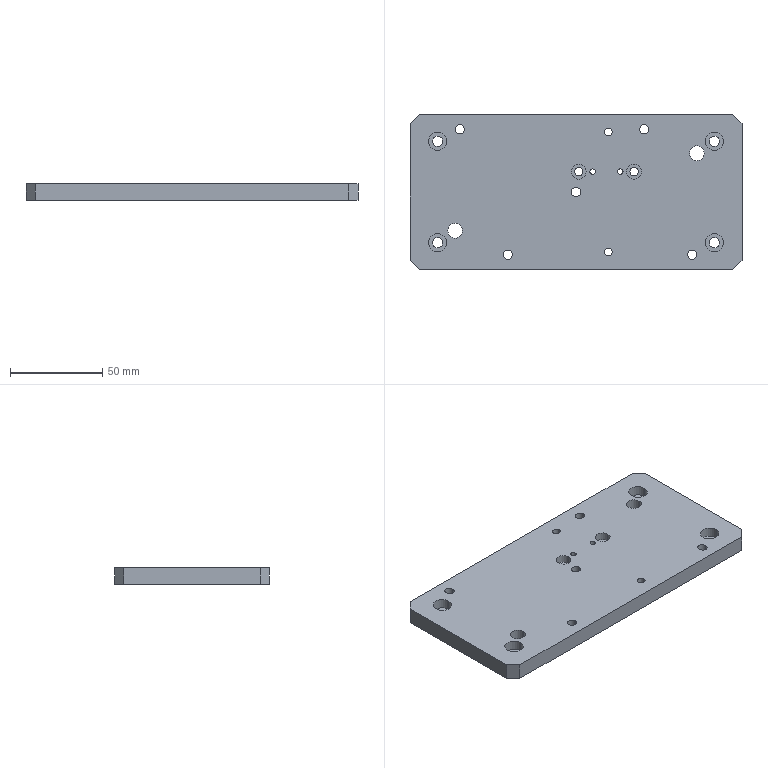Part | STEP file | PN_0010 | 1 solid | 62 faces | box 180 x 84 x 9 mm | volume 130838 mm3 | cylinder 46 | plane 16 | commonest cylinder face diameters 5 x10 5.5 x8 8 x8 10 x8 3 x4 4.2 x4